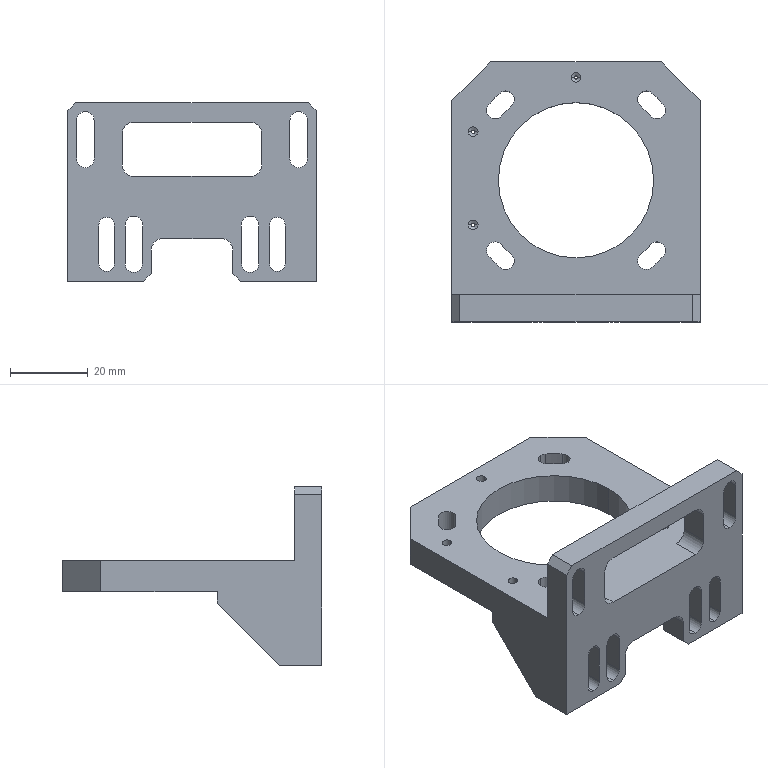NC program | NX | posted with a generic post | part box 64 x 67 x 46 mm
Lines 14132 to 14898 of 33790:
(ZLEVEL_PROFILE_COPY_1 , TOOL : D3)
N28226 T03 M6
N28228 G54
N28230 G17 G0 G90 X22.016 Y19.005 B0. C0. S5500 M3
N28232 G43 Z30. H3
N28234 Z-18.2
N28236 G94 G1 X22.802 Y18.185 Z-18.26 F1000.
N28238 X23.361 Y17.542 Z-18.304
N28240 X23.625 Y17.406 Z-18.32
N28242 X23.922 Y17.389 Z-18.335
N28244 X24.199 Y17.496 Z-18.351
N28246 X24.374 Y17.657 Z-18.363
N28248 X24.498 Y17.912 Z-18.378
N28250 X24.514 Y18.194 Z-18.393
N28252 X24.417 Y18.46 Z-18.408
N28254 X23.846 Y19.118 Z-18.454
N28256 X23.001 Y20.001 Z-18.518
N28258 X22.118 Y20.846 Z-18.582
N28260 X21.46 Y21.417 Z-18.627
N28262 X21.203 Y21.512 Z-18.642
N28264 X20.966 Y21.51 Z-18.654
N28266 X20.705 Y21.407 Z-18.669
N28268 X20.53 Y21.247 Z-18.681
N28270 X20.397 Y20.96 Z-18.698
N28272 X20.401 Y20.644 Z-18.714
N28274 X20.542 Y20.361 Z-18.731
N28276 X21.185 Y19.802 Z-18.776
N28278 X22.011 Y19.011 Z-18.836
N28280 X22.802 Y18.185 Z-18.895
N28282 X23.361 Y17.542 Z-18.94
N28284 X23.625 Y17.406 Z-18.956
N28286 X23.922 Y17.389 Z-18.971
N28288 X24.199 Y17.496 Z-18.987
N28290 X24.374 Y17.657 Z-18.999
N28292 X24.498 Y17.912 Z-19.014
N28294 X24.514 Y18.194 Z-19.029
N28296 X24.417 Y18.46 Z-19.044
N28298 X24.339 Y18.55 Z-19.05
N28300 G3 X21.55 Y21.339 R28.275 F1250.
N28302 X20.563 Y21.27 R0.7
N28304 X20.632 Y20.283 R0.7
N28306 G2 X23.283 Y17.632 R26.875
N28308 G3 X24.27 Y17.563 R0.7
N28310 X24.339 Y18.55 R0.7
N28312 G1 X24.26 Y18.639 Z-19.052
N28314 X24.179 Y18.727 Z-19.054
N28316 X24.099 Y18.815 Z-19.056
N28318 X24.019 Y18.904 Z-19.058
N28320 X23.939 Y18.992 Z-19.06
N28322 X23.857 Y19.079 Z-19.063
N28324 X23.778 Y19.168 Z-19.065
N28326 X23.697 Y19.256 Z-19.067
N28328 X23.617 Y19.345 Z-19.069
N28330 X23.536 Y19.433 Z-19.071
N28332 X23.455 Y19.521 Z-19.073
N28334 X23.371 Y19.605 Z-19.075
N28336 X23.287 Y19.69 Z-19.077
N28338 X23.202 Y19.774 Z-19.079
N28340 X23.119 Y19.859 Z-19.081
N28342 X23.033 Y19.943 Z-19.083
N28344 X22.95 Y20.028 Z-19.085
N28346 X22.866 Y20.112 Z-19.088
N28348 X22.781 Y20.196 Z-19.09
N28350 X22.697 Y20.281 Z-19.092
N28352 X22.612 Y20.365 Z-19.094
N28354 X22.527 Y20.449 Z-19.096
N28356 X22.44 Y20.53 Z-19.098
N28358 X22.354 Y20.613 Z-19.1
N28360 G3 X21.55 Y21.339 R28.275
N28362 X20.563 Y21.27 R0.7
N28364 X20.632 Y20.283 R0.7
N28366 G2 X23.283 Y17.632 R26.875
N28368 G3 X24.27 Y17.563 R0.7
N28370 X24.339 Y18.55 R0.7
N28372 G1 X24.26 Y18.639 Z-19.102
N28374 X24.179 Y18.727 Z-19.104
N28376 X24.099 Y18.815 Z-19.106
N28378 X24.019 Y18.904 Z-19.108
N28380 X23.939 Y18.992 Z-19.11
N28382 X23.857 Y19.079 Z-19.113
N28384 X23.778 Y19.168 Z-19.115
N28386 X23.697 Y19.256 Z-19.117
N28388 X23.617 Y19.345 Z-19.119
N28390 X23.536 Y19.433 Z-19.121
N28392 X23.455 Y19.521 Z-19.123
N28394 X23.371 Y19.605 Z-19.125
N28396 X23.287 Y19.69 Z-19.127
N28398 X23.202 Y19.774 Z-19.129
N28400 X23.119 Y19.859 Z-19.131
N28402 X23.033 Y19.943 Z-19.133
N28404 X22.95 Y20.028 Z-19.135
N28406 X22.866 Y20.112 Z-19.138
N28408 X22.781 Y20.196 Z-19.14
N28410 X22.697 Y20.281 Z-19.142
N28412 X22.612 Y20.365 Z-19.144
N28414 X22.527 Y20.449 Z-19.146
N28416 X22.44 Y20.53 Z-19.148
N28418 X22.354 Y20.613 Z-19.15
N28420 G3 X21.55 Y21.339 R28.275
N28422 X20.563 Y21.27 R0.7
N28424 X20.632 Y20.283 R0.7
N28426 G2 X23.283 Y17.632 R26.875
N28428 G3 X24.27 Y17.563 R0.7
N28430 X24.339 Y18.55 R0.7
N28432 G1 X24.26 Y18.639 Z-19.152
N28434 X24.179 Y18.727 Z-19.154
N28436 X24.099 Y18.815 Z-19.156
N28438 X24.019 Y18.904 Z-19.158
N28440 X23.939 Y18.992 Z-19.16
N28442 X23.857 Y19.079 Z-19.163
N28444 X23.778 Y19.168 Z-19.165
N28446 X23.697 Y19.256 Z-19.167
N28448 X23.617 Y19.345 Z-19.169
N28450 X23.536 Y19.433 Z-19.171
N28452 X23.455 Y19.521 Z-19.173
N28454 X23.371 Y19.605 Z-19.175
N28456 X23.287 Y19.69 Z-19.177
N28458 X23.202 Y19.774 Z-19.179
N28460 X23.119 Y19.859 Z-19.181
N28462 X23.033 Y19.943 Z-19.183
N28464 X22.95 Y20.028 Z-19.185
N28466 X22.866 Y20.112 Z-19.188
N28468 X22.781 Y20.196 Z-19.19
N28470 X22.696 Y20.281 Z-19.192
N28472 X22.612 Y20.365 Z-19.194
N28474 X22.527 Y20.449 Z-19.196
N28476 X22.44 Y20.53 Z-19.198
N28478 X22.354 Y20.613 Z-19.2
N28480 G3 X21.55 Y21.339 R28.275
N28482 X20.563 Y21.27 R0.7
N28484 X20.632 Y20.283 R0.7
N28486 G2 X23.283 Y17.632 R26.875
N28488 G3 X24.27 Y17.563 R0.7
N28490 X24.339 Y18.55 R0.7
N28492 G1 X24.26 Y18.639 Z-19.202
N28494 X24.179 Y18.727 Z-19.204
N28496 X24.099 Y18.815 Z-19.206
N28498 X24.019 Y18.904 Z-19.208
N28500 X23.939 Y18.992 Z-19.21
N28502 X23.857 Y19.079 Z-19.213
N28504 X23.778 Y19.168 Z-19.215
N28506 X23.697 Y19.256 Z-19.217
N28508 X23.617 Y19.345 Z-19.219
N28510 X23.536 Y19.433 Z-19.221
N28512 X23.455 Y19.521 Z-19.223
N28514 X23.371 Y19.605 Z-19.225
N28516 X23.287 Y19.69 Z-19.227
N28518 X23.202 Y19.774 Z-19.229
N28520 X23.119 Y19.859 Z-19.231
N28522 X23.033 Y19.943 Z-19.233
N28524 X22.95 Y20.028 Z-19.235
N28526 X22.866 Y20.112 Z-19.238
N28528 X22.781 Y20.196 Z-19.24
N28530 X22.696 Y20.281 Z-19.242
N28532 X22.612 Y20.365 Z-19.244
N28534 X22.527 Y20.449 Z-19.246
N28536 X22.44 Y20.53 Z-19.248
N28538 X22.354 Y20.613 Z-19.25
N28540 G3 X21.55 Y21.339 R28.275
N28542 X20.563 Y21.27 R0.7
N28544 X20.632 Y20.283 R0.7
N28546 G2 X23.283 Y17.632 R26.875
N28548 G3 X24.27 Y17.563 R0.7
N28550 X24.339 Y18.55 R0.7
N28552 G1 X24.26 Y18.639 Z-19.252
N28554 X24.179 Y18.727 Z-19.254
N28556 X24.099 Y18.815 Z-19.256
N28558 X24.019 Y18.904 Z-19.258
N28560 X23.939 Y18.992 Z-19.26
N28562 X23.857 Y19.079 Z-19.263
N28564 X23.778 Y19.168 Z-19.265
N28566 X23.697 Y19.256 Z-19.267
N28568 X23.617 Y19.345 Z-19.269
N28570 X23.536 Y19.433 Z-19.271
N28572 X23.455 Y19.521 Z-19.273
N28574 X23.371 Y19.605 Z-19.275
N28576 X23.287 Y19.69 Z-19.277
N28578 X23.202 Y19.774 Z-19.279
N28580 X23.119 Y19.859 Z-19.281
N28582 X23.033 Y19.943 Z-19.283
N28584 X22.95 Y20.028 Z-19.285
N28586 X22.866 Y20.112 Z-19.288
N28588 X22.781 Y20.196 Z-19.29
N28590 X22.696 Y20.281 Z-19.292
N28592 X22.612 Y20.365 Z-19.294
N28594 X22.527 Y20.449 Z-19.296
N28596 X22.44 Y20.53 Z-19.298
N28598 X22.354 Y20.613 Z-19.3
N28600 G3 X21.55 Y21.339 R28.275
N28602 X20.563 Y21.27 R0.7
N28604 X20.632 Y20.283 R0.7
N28606 G2 X23.283 Y17.632 R26.875
N28608 G3 X24.27 Y17.563 R0.7
N28610 X24.339 Y18.55 R0.7
N28612 G1 X24.26 Y18.639 Z-19.302
N28614 X24.179 Y18.727 Z-19.304
N28616 X24.099 Y18.815 Z-19.306
N28618 X24.019 Y18.904 Z-19.308
N28620 X23.939 Y18.992 Z-19.31
N28622 X23.857 Y19.079 Z-19.313
N28624 X23.778 Y19.168 Z-19.315
N28626 X23.697 Y19.256 Z-19.317
N28628 X23.617 Y19.345 Z-19.319
N28630 X23.536 Y19.433 Z-19.321
N28632 X23.455 Y19.521 Z-19.323
N28634 X23.371 Y19.605 Z-19.325
N28636 X23.287 Y19.69 Z-19.327
N28638 X23.202 Y19.774 Z-19.329
N28640 X23.119 Y19.859 Z-19.331
N28642 X23.033 Y19.943 Z-19.333
N28644 X22.95 Y20.028 Z-19.335
N28646 X22.866 Y20.112 Z-19.338
N28648 X22.781 Y20.196 Z-19.34
N28650 X22.696 Y20.281 Z-19.342
N28652 X22.612 Y20.365 Z-19.344
N28654 X22.527 Y20.449 Z-19.346
N28656 X22.44 Y20.53 Z-19.348
N28658 X22.354 Y20.613 Z-19.35
N28660 G3 X21.55 Y21.339 R28.275
N28662 X20.563 Y21.27 R0.7
N28664 X20.632 Y20.283 R0.7
N28666 G2 X23.283 Y17.632 R26.875
N28668 G3 X24.27 Y17.563 R0.7
N28670 X24.339 Y18.55 R0.7
N28672 G1 X24.26 Y18.639 Z-19.352
N28674 X24.179 Y18.727 Z-19.354
N28676 X24.099 Y18.815 Z-19.356
N28678 X24.019 Y18.904 Z-19.358
N28680 X23.938 Y18.992 Z-19.36
N28682 X23.857 Y19.079 Z-19.363
N28684 X23.778 Y19.168 Z-19.365
N28686 X23.697 Y19.256 Z-19.367
N28688 X23.617 Y19.345 Z-19.369
N28690 X23.536 Y19.433 Z-19.371
N28692 X23.455 Y19.521 Z-19.373
N28694 X23.371 Y19.605 Z-19.375
N28696 X23.287 Y19.69 Z-19.377
N28698 X23.202 Y19.774 Z-19.379
N28700 X23.119 Y19.859 Z-19.381
N28702 X23.033 Y19.943 Z-19.383
N28704 X22.95 Y20.028 Z-19.385
N28706 X22.866 Y20.112 Z-19.388
N28708 X22.781 Y20.196 Z-19.39
N28710 X22.696 Y20.281 Z-19.392
N28712 X22.612 Y20.365 Z-19.394
N28714 X22.527 Y20.449 Z-19.396
N28716 X22.44 Y20.53 Z-19.398
N28718 X22.354 Y20.613 Z-19.4
N28720 G3 X21.55 Y21.339 R28.275
N28722 X20.563 Y21.27 R0.7
N28724 X20.632 Y20.283 R0.7
N28726 G2 X23.283 Y17.632 R26.875
N28728 G3 X24.27 Y17.563 R0.7
N28730 X24.339 Y18.55 R0.7
N28732 G1 X24.26 Y18.639 Z-19.402
N28734 X24.179 Y18.727 Z-19.404
N28736 X24.099 Y18.815 Z-19.406
N28738 X24.019 Y18.904 Z-19.408
N28740 X23.938 Y18.992 Z-19.41
N28742 X23.857 Y19.079 Z-19.413
N28744 X23.778 Y19.168 Z-19.415
N28746 X23.697 Y19.256 Z-19.417
N28748 X23.617 Y19.345 Z-19.419
N28750 X23.536 Y19.433 Z-19.421
N28752 X23.455 Y19.521 Z-19.423
N28754 X23.371 Y19.605 Z-19.425
N28756 X23.287 Y19.69 Z-19.427
N28758 X23.202 Y19.774 Z-19.429
N28760 X23.119 Y19.859 Z-19.431
N28762 X23.033 Y19.943 Z-19.433
N28764 X22.95 Y20.028 Z-19.435
N28766 X22.866 Y20.112 Z-19.438
N28768 X22.781 Y20.196 Z-19.44
N28770 X22.696 Y20.281 Z-19.442
N28772 X22.612 Y20.365 Z-19.444
N28774 X22.527 Y20.449 Z-19.446
N28776 X22.44 Y20.53 Z-19.448
N28778 X22.354 Y20.613 Z-19.45
N28780 G3 X21.55 Y21.339 R28.275
N28782 X20.563 Y21.27 R0.7
N28784 X20.632 Y20.283 R0.7
N28786 G2 X23.283 Y17.632 R26.875
N28788 G3 X24.27 Y17.563 R0.7
N28790 X24.339 Y18.55 R0.7
N28792 G1 X24.26 Y18.639 Z-19.452
N28794 X24.179 Y18.727 Z-19.454
N28796 X24.099 Y18.815 Z-19.456
N28798 X24.019 Y18.904 Z-19.458
N28800 X23.938 Y18.992 Z-19.46
N28802 X23.857 Y19.079 Z-19.463
N28804 X23.778 Y19.168 Z-19.465
N28806 X23.697 Y19.256 Z-19.467
N28808 X23.617 Y19.345 Z-19.469
N28810 X23.536 Y19.433 Z-19.471
N28812 X23.455 Y19.521 Z-19.473
N28814 X23.371 Y19.605 Z-19.475
N28816 X23.287 Y19.69 Z-19.477
N28818 X23.202 Y19.774 Z-19.479
N28820 X23.119 Y19.859 Z-19.481
N28822 X23.033 Y19.943 Z-19.483
N28824 X22.95 Y20.028 Z-19.485
N28826 X22.866 Y20.112 Z-19.488
N28828 X22.781 Y20.196 Z-19.49
N28830 X22.696 Y20.281 Z-19.492
N28832 X22.612 Y20.365 Z-19.494
N28834 X22.527 Y20.449 Z-19.496
N28836 X22.44 Y20.53 Z-19.498
N28838 X22.354 Y20.613 Z-19.5
N28840 G3 X21.55 Y21.339 R28.275
N28842 X20.563 Y21.27 R0.7
N28844 X20.632 Y20.283 R0.7
N28846 G2 X23.283 Y17.632 R26.875
N28848 G3 X24.27 Y17.563 R0.7
N28850 X24.339 Y18.55 R0.7
N28852 G1 X24.26 Y18.639 Z-19.502
N28854 X24.179 Y18.727 Z-19.504
N28856 X24.099 Y18.815 Z-19.506
N28858 X24.019 Y18.904 Z-19.508
N28860 X23.938 Y18.992 Z-19.51
N28862 X23.857 Y19.079 Z-19.513
N28864 X23.778 Y19.168 Z-19.515
N28866 X23.697 Y19.256 Z-19.517
N28868 X23.617 Y19.345 Z-19.519
N28870 X23.536 Y19.433 Z-19.521
N28872 X23.455 Y19.521 Z-19.523
N28874 X23.371 Y19.605 Z-19.525
N28876 X23.287 Y19.69 Z-19.527
N28878 X23.202 Y19.774 Z-19.529
N28880 X23.118 Y19.859 Z-19.531
N28882 X23.033 Y19.943 Z-19.533
N28884 X22.95 Y20.028 Z-19.535
N28886 X22.866 Y20.112 Z-19.538
N28888 X22.781 Y20.196 Z-19.54
N28890 X22.696 Y20.281 Z-19.542
N28892 X22.612 Y20.365 Z-19.544
N28894 X22.527 Y20.449 Z-19.546
N28896 X22.44 Y20.53 Z-19.548
N28898 X22.354 Y20.613 Z-19.55
N28900 G3 X21.55 Y21.339 R28.275
N28902 X20.563 Y21.27 R0.7
N28904 X20.632 Y20.283 R0.7
N28906 G2 X23.283 Y17.632 R26.875
N28908 G3 X24.27 Y17.563 R0.7
N28910 X24.339 Y18.55 R0.7
N28912 G1 X24.26 Y18.639 Z-19.552
N28914 X24.179 Y18.727 Z-19.554
N28916 X24.099 Y18.815 Z-19.556
N28918 X24.019 Y18.904 Z-19.558
N28920 X23.938 Y18.992 Z-19.56
N28922 X23.857 Y19.079 Z-19.563
N28924 X23.778 Y19.168 Z-19.565
N28926 X23.697 Y19.256 Z-19.567
N28928 X23.617 Y19.345 Z-19.569
N28930 X23.536 Y19.433 Z-19.571
N28932 X23.455 Y19.521 Z-19.573
N28934 X23.371 Y19.605 Z-19.575
N28936 X23.287 Y19.69 Z-19.577
N28938 X23.202 Y19.774 Z-19.579
N28940 X23.118 Y19.859 Z-19.581
N28942 X23.033 Y19.943 Z-19.583
N28944 X22.95 Y20.028 Z-19.585
N28946 X22.866 Y20.112 Z-19.588
N28948 X22.781 Y20.196 Z-19.59
N28950 X22.696 Y20.281 Z-19.592
N28952 X22.612 Y20.365 Z-19.594
N28954 X22.527 Y20.449 Z-19.596
N28956 X22.44 Y20.53 Z-19.598
N28958 X22.354 Y20.613 Z-19.6
N28960 G3 X21.55 Y21.339 R28.275
N28962 X20.563 Y21.27 R0.7
N28964 X20.632 Y20.283 R0.7
N28966 G2 X23.283 Y17.632 R26.875
N28968 G3 X24.27 Y17.563 R0.7
N28970 X24.339 Y18.55 R0.7
N28972 G1 X24.26 Y18.639 Z-19.602
N28974 X24.179 Y18.727 Z-19.604
N28976 X24.099 Y18.815 Z-19.606
N28978 X24.019 Y18.904 Z-19.608
N28980 X23.938 Y18.992 Z-19.61
N28982 X23.857 Y19.079 Z-19.613
N28984 X23.778 Y19.168 Z-19.615
N28986 X23.697 Y19.256 Z-19.617
N28988 X23.617 Y19.345 Z-19.619
N28990 X23.536 Y19.433 Z-19.621
N28992 X23.455 Y19.521 Z-19.623
N28994 X23.371 Y19.605 Z-19.625
N28996 X23.287 Y19.69 Z-19.627
N28998 X23.202 Y19.774 Z-19.629
N29000 X23.118 Y19.859 Z-19.631
N29002 X23.033 Y19.943 Z-19.633
N29004 X22.95 Y20.028 Z-19.635
N29006 X22.866 Y20.112 Z-19.638
N29008 X22.781 Y20.196 Z-19.64
N29010 X22.696 Y20.281 Z-19.642
N29012 X22.612 Y20.365 Z-19.644
N29014 X22.527 Y20.449 Z-19.646
N29016 X22.44 Y20.53 Z-19.648
N29018 X22.354 Y20.613 Z-19.65
N29020 G3 X21.55 Y21.339 R28.275
N29022 X20.563 Y21.27 R0.7
N29024 X20.632 Y20.283 R0.7
N29026 G2 X23.283 Y17.632 R26.875
N29028 G3 X24.27 Y17.563 R0.7
N29030 X24.339 Y18.55 R0.7
N29032 G1 X24.26 Y18.639 Z-19.652
N29034 X24.179 Y18.727 Z-19.654
N29036 X24.099 Y18.815 Z-19.656
N29038 X24.019 Y18.904 Z-19.658
N29040 X23.938 Y18.992 Z-19.66
N29042 X23.857 Y19.079 Z-19.663
N29044 X23.777 Y19.168 Z-19.665
N29046 X23.697 Y19.256 Z-19.667
N29048 X23.617 Y19.345 Z-19.669
N29050 X23.536 Y19.433 Z-19.671
N29052 X23.455 Y19.521 Z-19.673
N29054 X23.371 Y19.605 Z-19.675
N29056 X23.287 Y19.69 Z-19.677
N29058 X23.202 Y19.774 Z-19.679
N29060 X23.118 Y19.859 Z-19.681
N29062 X23.033 Y19.943 Z-19.683
N29064 X22.95 Y20.028 Z-19.685
N29066 X22.866 Y20.112 Z-19.688
N29068 X22.781 Y20.196 Z-19.69
N29070 X22.696 Y20.281 Z-19.692
N29072 X22.612 Y20.365 Z-19.694
N29074 X22.527 Y20.449 Z-19.696
N29076 X22.44 Y20.53 Z-19.698
N29078 X22.354 Y20.613 Z-19.7
N29080 G3 X21.55 Y21.339 R28.275
N29082 X20.563 Y21.27 R0.7
N29084 X20.632 Y20.283 R0.7
N29086 G2 X23.283 Y17.632 R26.875
N29088 G3 X24.27 Y17.563 R0.7
N29090 X24.339 Y18.55 R0.7
N29092 G1 X24.26 Y18.639 Z-19.702
N29094 X24.179 Y18.727 Z-19.704
N29096 X24.099 Y18.815 Z-19.706
N29098 X24.019 Y18.904 Z-19.708
N29100 X23.938 Y18.992 Z-19.71
N29102 X23.857 Y19.079 Z-19.713
N29104 X23.777 Y19.168 Z-19.715
N29106 X23.697 Y19.256 Z-19.717
N29108 X23.617 Y19.345 Z-19.719
N29110 X23.536 Y19.433 Z-19.721
N29112 X23.455 Y19.521 Z-19.723
N29114 X23.371 Y19.605 Z-19.725
N29116 X23.287 Y19.69 Z-19.727
N29118 X23.202 Y19.774 Z-19.729
N29120 X23.118 Y19.859 Z-19.731
N29122 X23.033 Y19.943 Z-19.733
N29124 X22.95 Y20.028 Z-19.735
N29126 X22.866 Y20.112 Z-19.738
N29128 X22.781 Y20.196 Z-19.74
N29130 X22.696 Y20.281 Z-19.742
N29132 X22.612 Y20.365 Z-19.744
N29134 X22.527 Y20.449 Z-19.746
N29136 X22.44 Y20.53 Z-19.748
N29138 X22.354 Y20.613 Z-19.75
N29140 G3 X21.55 Y21.339 R28.275
N29142 X20.563 Y21.27 R0.7
N29144 X20.632 Y20.283 R0.7
N29146 G2 X23.283 Y17.632 R26.875
N29148 G3 X24.27 Y17.563 R0.7
N29150 X24.339 Y18.55 R0.7
N29152 G1 X24.26 Y18.639 Z-19.752
N29154 X24.179 Y18.727 Z-19.754
N29156 X24.099 Y18.815 Z-19.756
N29158 X24.019 Y18.904 Z-19.758
N29160 X23.938 Y18.992 Z-19.76
N29162 X23.857 Y19.079 Z-19.763
N29164 X23.777 Y19.168 Z-19.765
N29166 X23.697 Y19.256 Z-19.767
N29168 X23.617 Y19.345 Z-19.769
N29170 X23.536 Y19.433 Z-19.771
N29172 X23.455 Y19.521 Z-19.773
N29174 X23.371 Y19.605 Z-19.775
N29176 X23.287 Y19.69 Z-19.777
N29178 X23.202 Y19.774 Z-19.779
N29180 X23.118 Y19.859 Z-19.781
N29182 X23.033 Y19.943 Z-19.783
N29184 X22.95 Y20.028 Z-19.785
N29186 X22.866 Y20.112 Z-19.788
N29188 X22.781 Y20.196 Z-19.79
N29190 X22.696 Y20.281 Z-19.792
N29192 X22.612 Y20.365 Z-19.794
N29194 X22.527 Y20.449 Z-19.796
N29196 X22.44 Y20.53 Z-19.798
N29198 X22.354 Y20.613 Z-19.8
N29200 G3 X21.55 Y21.339 R28.275
N29202 X20.563 Y21.27 R0.7
N29204 X20.632 Y20.283 R0.7
N29206 G2 X23.283 Y17.632 R26.875
N29208 G3 X24.27 Y17.563 R0.7
N29210 X24.339 Y18.55 R0.7
N29212 G1 X24.26 Y18.639 Z-19.802
N29214 X24.179 Y18.727 Z-19.804
N29216 X24.099 Y18.815 Z-19.806
N29218 X24.019 Y18.904 Z-19.808
N29220 X23.938 Y18.992 Z-19.81
N29222 X23.857 Y19.079 Z-19.813
N29224 X23.777 Y19.168 Z-19.815
N29226 X23.697 Y19.256 Z-19.817
N29228 X23.617 Y19.345 Z-19.819
N29230 X23.536 Y19.433 Z-19.821
N29232 X23.455 Y19.521 Z-19.823
N29234 X23.371 Y19.605 Z-19.825
N29236 X23.287 Y19.69 Z-19.827
N29238 X23.202 Y19.774 Z-19.829
N29240 X23.118 Y19.859 Z-19.831
N29242 X23.033 Y19.943 Z-19.833
N29244 X22.95 Y20.028 Z-19.835
N29246 X22.866 Y20.112 Z-19.838
N29248 X22.781 Y20.196 Z-19.84
N29250 X22.696 Y20.281 Z-19.842
N29252 X22.612 Y20.365 Z-19.844
N29254 X22.527 Y20.449 Z-19.846
N29256 X22.44 Y20.53 Z-19.848
N29258 X22.354 Y20.613 Z-19.85
N29260 G3 X21.55 Y21.339 R28.275
N29262 X20.563 Y21.27 R0.7
N29264 X20.632 Y20.283 R0.7
N29266 G2 X23.283 Y17.632 R26.875
N29268 G3 X24.27 Y17.563 R0.7
N29270 X24.339 Y18.55 R0.7
N29272 G1 X24.26 Y18.639 Z-19.852
N29274 X24.179 Y18.727 Z-19.854
N29276 X24.099 Y18.815 Z-19.856
N29278 X24.019 Y18.904 Z-19.858
N29280 X23.938 Y18.992 Z-19.86
N29282 X23.857 Y19.079 Z-19.863
N29284 X23.777 Y19.168 Z-19.865
N29286 X23.697 Y19.256 Z-19.867
N29288 X23.617 Y19.345 Z-19.869
N29290 X23.536 Y19.433 Z-19.871
N29292 X23.455 Y19.521 Z-19.873
N29294 X23.371 Y19.605 Z-19.875
N29296 X23.287 Y19.69 Z-19.877
N29298 X23.202 Y19.774 Z-19.879
N29300 X23.118 Y19.859 Z-19.881
N29302 X23.033 Y19.943 Z-19.883
N29304 X22.95 Y20.028 Z-19.885
N29306 X22.866 Y20.112 Z-19.888
N29308 X22.781 Y20.196 Z-19.89
N29310 X22.696 Y20.281 Z-19.892
N29312 X22.612 Y20.365 Z-19.894
N29314 X22.527 Y20.449 Z-19.896
N29316 X22.44 Y20.53 Z-19.898
N29318 X22.354 Y20.613 Z-19.9
N29320 G3 X21.55 Y21.339 R28.275
N29322 X20.563 Y21.27 R0.7
N29324 X20.632 Y20.283 R0.7
N29326 G2 X23.283 Y17.632 R26.875
N29328 G3 X24.27 Y17.563 R0.7
N29330 X24.339 Y18.55 R0.7
N29332 G1 X24.26 Y18.639 Z-19.902
N29334 X24.179 Y18.727 Z-19.904
N29336 X24.099 Y18.815 Z-19.906
N29338 X24.019 Y18.904 Z-19.908
N29340 X23.938 Y18.992 Z-19.91
N29342 X23.857 Y19.079 Z-19.913
N29344 X23.777 Y19.168 Z-19.915
N29346 X23.697 Y19.256 Z-19.917
N29348 X23.617 Y19.345 Z-19.919
N29350 X23.536 Y19.433 Z-19.921
N29352 X23.455 Y19.521 Z-19.923
N29354 X23.371 Y19.605 Z-19.925
N29356 X23.287 Y19.69 Z-19.927
N29358 X23.202 Y19.774 Z-19.929
N29360 X23.118 Y19.859 Z-19.931
N29362 X23.033 Y19.943 Z-19.933
N29364 X22.95 Y20.028 Z-19.935
N29366 X22.866 Y20.112 Z-19.938
N29368 X22.781 Y20.196 Z-19.94
N29370 X22.696 Y20.281 Z-19.942
N29372 X22.612 Y20.365 Z-19.944
N29374 X22.527 Y20.449 Z-19.946
N29376 X22.44 Y20.53 Z-19.948
N29378 X22.354 Y20.613 Z-19.95
N29380 G3 X21.55 Y21.339 R28.275
N29382 X20.563 Y21.27 R0.7
N29384 X20.632 Y20.283 R0.7
N29386 G2 X23.283 Y17.632 R26.875
N29388 G3 X24.27 Y17.563 R0.7
N29390 X24.339 Y18.55 R0.7
N29392 G1 X24.26 Y18.639 Z-19.952
N29394 X24.179 Y18.727 Z-19.954
N29396 X24.099 Y18.815 Z-19.956
N29398 X24.019 Y18.904 Z-19.958
N29400 X23.938 Y18.992 Z-19.96
N29402 X23.857 Y19.079 Z-19.963
N29404 X23.777 Y19.168 Z-19.965
N29406 X23.697 Y19.256 Z-19.967
N29408 X23.617 Y19.345 Z-19.969
N29410 X23.536 Y19.433 Z-19.971
N29412 X23.455 Y19.521 Z-19.973
N29414 X23.371 Y19.605 Z-19.975
N29416 X23.287 Y19.69 Z-19.977
N29418 X23.202 Y19.774 Z-19.979
N29420 X23.118 Y19.859 Z-19.981
N29422 X23.033 Y19.943 Z-19.983
N29424 X22.95 Y20.028 Z-19.985
N29426 X22.866 Y20.112 Z-19.988
N29428 X22.781 Y20.196 Z-19.99
N29430 X22.696 Y20.281 Z-19.992
N29432 X22.612 Y20.365 Z-19.994
N29434 X22.527 Y20.449 Z-19.996
N29436 X22.44 Y20.53 Z-19.998
N29438 X22.354 Y20.613 Z-20.
N29440 G3 X21.55 Y21.339 R28.275
N29442 X20.563 Y21.27 R0.7
N29444 X20.632 Y20.283 R0.7
N29446 G2 X23.283 Y17.632 R26.875
N29448 G3 X24.27 Y17.563 R0.7
N29450 X24.339 Y18.55 R0.7
N29452 G1 X24.26 Y18.639 Z-20.002
N29454 X24.179 Y18.727 Z-20.004
N29456 X24.099 Y18.815 Z-20.006
N29458 X24.019 Y18.904 Z-20.008
N29460 X23.938 Y18.992 Z-20.01
N29462 X23.857 Y19.079 Z-20.013
N29464 X23.777 Y19.168 Z-20.015
N29466 X23.697 Y19.256 Z-20.017
N29468 X23.617 Y19.345 Z-20.019
N29470 X23.536 Y19.433 Z-20.021
N29472 X23.455 Y19.521 Z-20.023
N29474 X23.371 Y19.605 Z-20.025
N29476 X23.287 Y19.69 Z-20.027
N29478 X23.202 Y19.774 Z-20.029
N29480 X23.118 Y19.859 Z-20.031
N29482 X23.033 Y19.943 Z-20.033
N29484 X22.95 Y20.028 Z-20.035
N29486 X22.866 Y20.112 Z-20.038
N29488 X22.781 Y20.196 Z-20.04
N29490 X22.696 Y20.281 Z-20.042
N29492 X22.612 Y20.365 Z-20.044
N29494 X22.527 Y20.449 Z-20.046
N29496 X22.44 Y20.53 Z-20.048
N29498 X22.354 Y20.613 Z-20.05
N29500 G3 X21.55 Y21.339 R28.275
N29502 X20.563 Y21.27 R0.7
N29504 X20.632 Y20.283 R0.7
N29506 G2 X23.283 Y17.632 R26.875
N29508 G3 X24.27 Y17.563 R0.7
N29510 X24.339 Y18.55 R0.7
N29512 G1 X24.26 Y18.639 Z-20.052
N29514 X24.179 Y18.727 Z-20.054
N29516 X24.099 Y18.815 Z-20.056
N29518 X24.019 Y18.904 Z-20.058
N29520 X23.938 Y18.992 Z-20.06
N29522 X23.857 Y19.079 Z-20.063
N29524 X23.777 Y19.168 Z-20.065
N29526 X23.697 Y19.256 Z-20.067
N29528 X23.617 Y19.345 Z-20.069
N29530 X23.536 Y19.433 Z-20.071
N29532 X23.455 Y19.521 Z-20.073
N29534 X23.371 Y19.605 Z-20.075
N29536 X23.287 Y19.69 Z-20.077
N29538 X23.202 Y19.774 Z-20.079
N29540 X23.118 Y19.859 Z-20.081
N29542 X23.033 Y19.943 Z-20.083
N29544 X22.95 Y20.028 Z-20.085
N29546 X22.866 Y20.112 Z-20.088
N29548 X22.781 Y20.196 Z-20.09
N29550 X22.696 Y20.281 Z-20.092
N29552 X22.612 Y20.365 Z-20.094
N29554 X22.527 Y20.449 Z-20.096
N29556 X22.44 Y20.53 Z-20.098
N29558 X22.354 Y20.613 Z-20.1
N29560 G3 X21.55 Y21.339 R28.275
N29562 X20.563 Y21.27 R0.7
N29564 X20.632 Y20.283 R0.7
N29566 G2 X23.283 Y17.632 R26.875
N29568 G3 X24.27 Y17.563 R0.7
N29570 X24.339 Y18.55 R0.7
N29572 G1 X24.26 Y18.639 Z-20.102
N29574 X24.179 Y18.727 Z-20.104
N29576 X24.099 Y18.815 Z-20.106
N29578 X24.019 Y18.904 Z-20.108
N29580 X23.938 Y18.992 Z-20.11
N29582 X23.857 Y19.079 Z-20.113
N29584 X23.777 Y19.168 Z-20.115
N29586 X23.697 Y19.256 Z-20.117
N29588 X23.617 Y19.345 Z-20.119
N29590 X23.536 Y19.433 Z-20.121
N29592 X23.455 Y19.521 Z-20.123
N29594 X23.371 Y19.605 Z-20.125
N29596 X23.287 Y19.69 Z-20.127
N29598 X23.202 Y19.774 Z-20.129
N29600 X23.118 Y19.859 Z-20.131
N29602 X23.033 Y19.943 Z-20.133
N29604 X22.95 Y20.028 Z-20.135
N29606 X22.866 Y20.112 Z-20.138
N29608 X22.781 Y20.196 Z-20.14
N29610 X22.696 Y20.281 Z-20.142
N29612 X22.612 Y20.365 Z-20.144
N29614 X22.527 Y20.449 Z-20.146
N29616 X22.44 Y20.53 Z-20.148
N29618 X22.354 Y20.613 Z-20.15
N29620 G3 X21.55 Y21.339 R28.275
N29622 X20.563 Y21.27 R0.7
N29624 X20.632 Y20.283 R0.7
N29626 G2 X23.283 Y17.632 R26.875
N29628 G3 X24.27 Y17.563 R0.7
N29630 X24.339 Y18.55 R0.7
N29632 G1 X24.26 Y18.639 Z-20.152
N29634 X24.179 Y18.727 Z-20.154
N29636 X24.099 Y18.815 Z-20.156
N29638 X24.019 Y18.904 Z-20.158
N29640 X23.938 Y18.992 Z-20.16
N29642 X23.857 Y19.079 Z-20.163
N29644 X23.777 Y19.168 Z-20.165
N29646 X23.697 Y19.256 Z-20.167
N29648 X23.617 Y19.345 Z-20.169
N29650 X23.536 Y19.433 Z-20.171
N29652 X23.455 Y19.521 Z-20.173
N29654 X23.371 Y19.605 Z-20.175
N29656 X23.287 Y19.69 Z-20.177
N29658 X23.202 Y19.774 Z-20.179
N29660 X23.118 Y19.859 Z-20.181
N29662 X23.033 Y19.943 Z-20.183
N29664 X22.95 Y20.028 Z-20.185
N29666 X22.866 Y20.112 Z-20.188
N29668 X22.781 Y20.196 Z-20.19
N29670 X22.696 Y20.281 Z-20.192
N29672 X22.612 Y20.365 Z-20.194
N29674 X22.527 Y20.449 Z-20.196
N29676 X22.44 Y20.53 Z-20.198
N29678 X22.354 Y20.613 Z-20.2
N29680 G3 X21.55 Y21.339 R28.275
N29682 X20.563 Y21.27 R0.7
N29684 X20.632 Y20.283 R0.7
N29686 G2 X23.283 Y17.632 R26.875
N29688 G3 X24.27 Y17.563 R0.7
N29690 X24.339 Y18.55 R0.7
N29692 G1 X24.26 Y18.639 Z-20.202
N29694 X24.179 Y18.727 Z-20.204
N29696 X24.099 Y18.815 Z-20.206
N29698 X24.019 Y18.904 Z-20.208
N29700 X23.938 Y18.992 Z-20.21
N29702 X23.857 Y19.079 Z-20.213
N29704 X23.777 Y19.168 Z-20.215
N29706 X23.697 Y19.256 Z-20.217
N29708 X23.617 Y19.345 Z-20.219
N29710 X23.536 Y19.433 Z-20.221
N29712 X23.455 Y19.521 Z-20.223
N29714 X23.371 Y19.605 Z-20.225
N29716 X23.287 Y19.69 Z-20.227
N29718 X23.202 Y19.774 Z-20.229
N29720 X23.118 Y19.859 Z-20.231
N29722 X23.033 Y19.943 Z-20.233
N29724 X22.95 Y20.028 Z-20.235
N29726 X22.866 Y20.112 Z-20.238
N29728 X22.781 Y20.196 Z-20.24
N29730 X22.696 Y20.281 Z-20.242
N29732 X22.612 Y20.365 Z-20.244
N29734 X22.527 Y20.449 Z-20.246
N29736 X22.44 Y20.53 Z-20.248
N29738 X22.354 Y20.613 Z-20.25
N29740 G3 X21.55 Y21.339 R28.275
N29742 X20.563 Y21.27 R0.7
N29744 X20.632 Y20.283 R0.7
N29746 G2 X23.283 Y17.632 R26.875
N29748 G3 X24.27 Y17.563 R0.7
N29750 X24.339 Y18.55 R0.7
N29752 G1 X24.26 Y18.639 Z-20.252